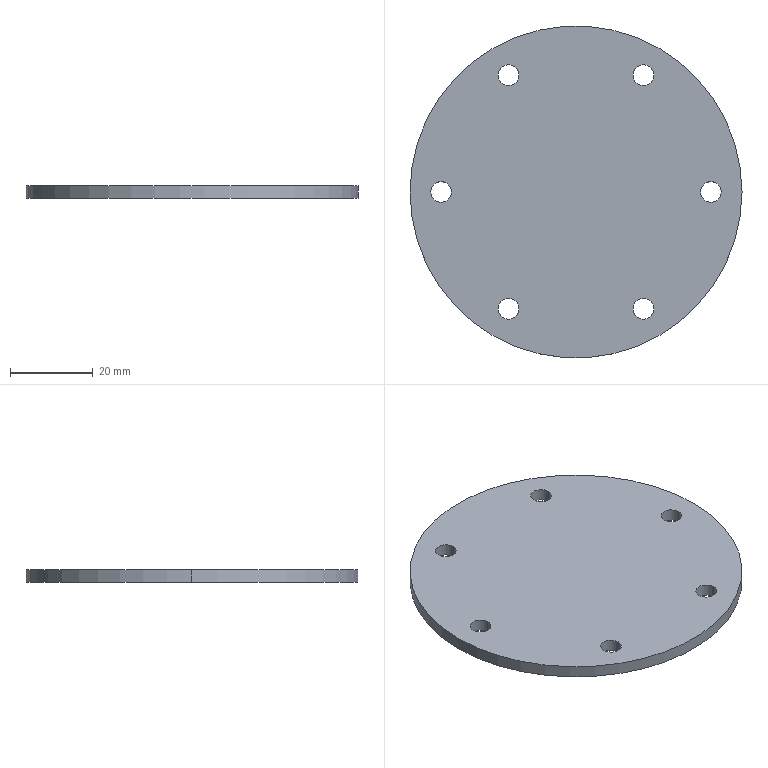Part | SolidWorks | features FlatPattern 1, SMBaseFlange 1, SheetMetal 1 | 1 solid | 16 faces | box 80 x 80 x 3 mm | volume 14726 mm3 | cylinder 14 | plane 2 | commonest cylinder face diameters 5 x12 80 x2
STEP:
#1=CARTESIAN_POINT('',(498.39,-36.604,3.));
#2=VERTEX_POINT('',#1);
#3=CARTESIAN_POINT('',(503.39,-36.604,3.));
#4=VERTEX_POINT('',#3);
#5=CARTESIAN_POINT('',(500.89,-36.604,3.));
#6=DIRECTION('',(0.,0.,1.));
#7=DIRECTION('',(1.,0.,0.));
#8=AXIS2_PLACEMENT_3D('',#5,#6,#7);
#9=CIRCLE('',#8,2.5);
#10=EDGE_CURVE('',#2,#4,#9,.T.);
#11=ORIENTED_EDGE('',*,*,#10,.T.);
#12=CARTESIAN_POINT('',(503.39,-36.604,0.));
#13=VERTEX_POINT('',#12);
#14=CARTESIAN_POINT('',(503.39,-36.604,3.));
#15=DIRECTION('',(0.,0.,-1.));
#16=VECTOR('',#15,1000.);
#17=LINE('',#14,#16);
#18=EDGE_CURVE('',#4,#13,#17,.T.);
#19=ORIENTED_EDGE('',*,*,#18,.T.);
#20=CARTESIAN_POINT('',(498.39,-36.604,0.));
#21=VERTEX_POINT('',#20);
#22=CARTESIAN_POINT('',(500.89,-36.604,0.));
#23=DIRECTION('',(0.,0.,1.));
#24=DIRECTION('',(1.,0.,0.));
#25=AXIS2_PLACEMENT_3D('',#22,#23,#24);
#26=CIRCLE('',#25,2.5);
#27=EDGE_CURVE('',#21,#13,#26,.T.);
#28=ORIENTED_EDGE('',*,*,#27,.F.);
#29=CARTESIAN_POINT('',(498.39,-36.604,3.));
#30=DIRECTION('',(0.,0.,-1.));
#31=VECTOR('',#30,1000.);
#32=LINE('',#29,#31);
#33=EDGE_CURVE('',#2,#21,#32,.T.);
#34=ORIENTED_EDGE('',*,*,#33,.F.);
#35=EDGE_LOOP('',(#11,#19,#28,#34));
#36=FACE_OUTER_BOUND('',#35,.T.);
#37=CARTESIAN_POINT('',(500.89,-36.604,3.));
#38=DIRECTION('',(0.,0.,-1.));
#39=DIRECTION('',(-1.,0.,0.));
#40=AXIS2_PLACEMENT_3D('',#37,#38,#39);
#41=CYLINDRICAL_SURFACE('',#40,2.5);
#42=ADVANCED_FACE('',(#36),#41,.F.);
#43=CARTESIAN_POINT('',(465.89,-36.604,3.));
#44=VERTEX_POINT('',#43);
#45=CARTESIAN_POINT('',(470.89,-36.604,3.));
#46=VERTEX_POINT('',#45);
#47=CARTESIAN_POINT('',(468.39,-36.604,3.));
#48=DIRECTION('',(0.,0.,1.));
#49=DIRECTION('',(1.,0.,0.));
#50=AXIS2_PLACEMENT_3D('',#47,#48,#49);
#51=CIRCLE('',#50,2.5);
#52=EDGE_CURVE('',#44,#46,#51,.T.);
#53=ORIENTED_EDGE('',*,*,#52,.T.);
#54=CARTESIAN_POINT('',(470.89,-36.604,0.));
#55=VERTEX_POINT('',#54);
#56=CARTESIAN_POINT('',(470.89,-36.604,3.));
#57=DIRECTION('',(0.,0.,-1.));
#58=VECTOR('',#57,1000.);
#59=LINE('',#56,#58);
#60=EDGE_CURVE('',#46,#55,#59,.T.);
#61=ORIENTED_EDGE('',*,*,#60,.T.);
#62=CARTESIAN_POINT('',(465.89,-36.604,0.));
#63=VERTEX_POINT('',#62);
#64=CARTESIAN_POINT('',(468.39,-36.604,0.));
#65=DIRECTION('',(0.,0.,1.));
#66=DIRECTION('',(1.,0.,0.));
#67=AXIS2_PLACEMENT_3D('',#64,#65,#66);
#68=CIRCLE('',#67,2.5);
#69=EDGE_CURVE('',#63,#55,#68,.T.);
#70=ORIENTED_EDGE('',*,*,#69,.F.);
#71=CARTESIAN_POINT('',(465.89,-36.604,3.));
#72=DIRECTION('',(0.,0.,-1.));
#73=VECTOR('',#72,1000.);
#74=LINE('',#71,#73);
#75=EDGE_CURVE('',#44,#63,#74,.T.);
#76=ORIENTED_EDGE('',*,*,#75,.F.);
#77=EDGE_LOOP('',(#53,#61,#70,#76));
#78=FACE_OUTER_BOUND('',#77,.T.);
#79=CARTESIAN_POINT('',(468.39,-36.604,3.));
#80=DIRECTION('',(0.,0.,-1.));
#81=DIRECTION('',(-1.,0.,0.));
#82=AXIS2_PLACEMENT_3D('',#79,#80,#81);
#83=CYLINDRICAL_SURFACE('',#82,2.5);
#84=ADVANCED_FACE('',(#78),#83,.F.);
#85=CARTESIAN_POINT('',(449.64,-64.75,3.));
#86=VERTEX_POINT('',#85);
#87=CARTESIAN_POINT('',(454.64,-64.75,3.));
#88=VERTEX_POINT('',#87);
#89=CARTESIAN_POINT('',(452.14,-64.75,3.));
#90=DIRECTION('',(0.,0.,1.));
#91=DIRECTION('',(1.,0.,0.));
#92=AXIS2_PLACEMENT_3D('',#89,#90,#91);
#93=CIRCLE('',#92,2.5);
#94=EDGE_CURVE('',#86,#88,#93,.T.);
#95=ORIENTED_EDGE('',*,*,#94,.T.);
#96=CARTESIAN_POINT('',(454.64,-64.75,0.));
#97=VERTEX_POINT('',#96);
#98=CARTESIAN_POINT('',(454.64,-64.75,3.));
#99=DIRECTION('',(0.,0.,-1.));
#100=VECTOR('',#99,1000.);
#101=LINE('',#98,#100);
#102=EDGE_CURVE('',#88,#97,#101,.T.);
#103=ORIENTED_EDGE('',*,*,#102,.T.);
#104=CARTESIAN_POINT('',(449.64,-64.75,0.));
#105=VERTEX_POINT('',#104);
#106=CARTESIAN_POINT('',(452.14,-64.75,0.));
#107=DIRECTION('',(0.,0.,1.));
#108=DIRECTION('',(1.,0.,0.));
#109=AXIS2_PLACEMENT_3D('',#106,#107,#108);
#110=CIRCLE('',#109,2.5);
#111=EDGE_CURVE('',#105,#97,#110,.T.);
#112=ORIENTED_EDGE('',*,*,#111,.F.);
#113=CARTESIAN_POINT('',(449.64,-64.75,3.));
#114=DIRECTION('',(0.,0.,-1.));
#115=VECTOR('',#114,1000.);
#116=LINE('',#113,#115);
#117=EDGE_CURVE('',#86,#105,#116,.T.);
#118=ORIENTED_EDGE('',*,*,#117,.F.);
#119=EDGE_LOOP('',(#95,#103,#112,#118));
#120=FACE_OUTER_BOUND('',#119,.T.);
#121=CARTESIAN_POINT('',(452.14,-64.75,3.));
#122=DIRECTION('',(0.,0.,-1.));
#123=DIRECTION('',(-1.,0.,0.));
#124=AXIS2_PLACEMENT_3D('',#121,#122,#123);
#125=CYLINDRICAL_SURFACE('',#124,2.5);
#126=ADVANCED_FACE('',(#120),#125,.F.);
#127=CARTESIAN_POINT('',(465.89,-92.896,3.));
#128=VERTEX_POINT('',#127);
#129=CARTESIAN_POINT('',(470.89,-92.896,3.));
#130=VERTEX_POINT('',#129);
#131=CARTESIAN_POINT('',(468.39,-92.896,3.));
#132=DIRECTION('',(0.,0.,1.));
#133=DIRECTION('',(1.,0.,0.));
#134=AXIS2_PLACEMENT_3D('',#131,#132,#133);
#135=CIRCLE('',#134,2.5);
#136=EDGE_CURVE('',#128,#130,#135,.T.);
#137=ORIENTED_EDGE('',*,*,#136,.T.);
#138=CARTESIAN_POINT('',(470.89,-92.896,0.));
#139=VERTEX_POINT('',#138);
#140=CARTESIAN_POINT('',(470.89,-92.896,3.));
#141=DIRECTION('',(0.,0.,-1.));
#142=VECTOR('',#141,1000.);
#143=LINE('',#140,#142);
#144=EDGE_CURVE('',#130,#139,#143,.T.);
#145=ORIENTED_EDGE('',*,*,#144,.T.);
#146=CARTESIAN_POINT('',(465.89,-92.896,0.));
#147=VERTEX_POINT('',#146);
#148=CARTESIAN_POINT('',(468.39,-92.896,0.));
#149=DIRECTION('',(0.,0.,1.));
#150=DIRECTION('',(1.,0.,0.));
#151=AXIS2_PLACEMENT_3D('',#148,#149,#150);
#152=CIRCLE('',#151,2.5);
#153=EDGE_CURVE('',#147,#139,#152,.T.);
#154=ORIENTED_EDGE('',*,*,#153,.F.);
#155=CARTESIAN_POINT('',(465.89,-92.896,3.));
#156=DIRECTION('',(0.,0.,-1.));
#157=VECTOR('',#156,1000.);
#158=LINE('',#155,#157);
#159=EDGE_CURVE('',#128,#147,#158,.T.);
#160=ORIENTED_EDGE('',*,*,#159,.F.);
#161=EDGE_LOOP('',(#137,#145,#154,#160));
#162=FACE_OUTER_BOUND('',#161,.T.);
#163=CARTESIAN_POINT('',(468.39,-92.896,3.));
#164=DIRECTION('',(0.,0.,-1.));
#165=DIRECTION('',(-1.,0.,0.));
#166=AXIS2_PLACEMENT_3D('',#163,#164,#165);
#167=CYLINDRICAL_SURFACE('',#166,2.5);
#168=ADVANCED_FACE('',(#162),#167,.F.);
#169=CARTESIAN_POINT('',(498.39,-92.896,3.));
#170=VERTEX_POINT('',#169);
#171=CARTESIAN_POINT('',(503.39,-92.896,3.));
#172=VERTEX_POINT('',#171);
#173=CARTESIAN_POINT('',(500.89,-92.896,3.));
#174=DIRECTION('',(0.,0.,1.));
#175=DIRECTION('',(1.,0.,0.));
#176=AXIS2_PLACEMENT_3D('',#173,#174,#175);
#177=CIRCLE('',#176,2.5);
#178=EDGE_CURVE('',#170,#172,#177,.T.);
#179=ORIENTED_EDGE('',*,*,#178,.T.);
#180=CARTESIAN_POINT('',(503.39,-92.896,0.));
#181=VERTEX_POINT('',#180);
#182=CARTESIAN_POINT('',(503.39,-92.896,3.));
#183=DIRECTION('',(0.,0.,-1.));
#184=VECTOR('',#183,1000.);
#185=LINE('',#182,#184);
#186=EDGE_CURVE('',#172,#181,#185,.T.);
#187=ORIENTED_EDGE('',*,*,#186,.T.);
#188=CARTESIAN_POINT('',(498.39,-92.896,0.));
#189=VERTEX_POINT('',#188);
#190=CARTESIAN_POINT('',(500.89,-92.896,0.));
#191=DIRECTION('',(0.,0.,1.));
#192=DIRECTION('',(1.,0.,0.));
#193=AXIS2_PLACEMENT_3D('',#190,#191,#192);
#194=CIRCLE('',#193,2.5);
#195=EDGE_CURVE('',#189,#181,#194,.T.);
#196=ORIENTED_EDGE('',*,*,#195,.F.);
#197=CARTESIAN_POINT('',(498.39,-92.896,3.));
#198=DIRECTION('',(0.,0.,-1.));
#199=VECTOR('',#198,1000.);
#200=LINE('',#197,#199);
#201=EDGE_CURVE('',#170,#189,#200,.T.);
#202=ORIENTED_EDGE('',*,*,#201,.F.);
#203=EDGE_LOOP('',(#179,#187,#196,#202));
#204=FACE_OUTER_BOUND('',#203,.T.);
#205=CARTESIAN_POINT('',(500.89,-92.896,3.));
#206=DIRECTION('',(0.,0.,-1.));
#207=DIRECTION('',(-1.,0.,0.));
#208=AXIS2_PLACEMENT_3D('',#205,#206,#207);
#209=CYLINDRICAL_SURFACE('',#208,2.5);
#210=ADVANCED_FACE('',(#204),#209,.F.);
#211=CARTESIAN_POINT('',(514.64,-64.75,3.));
#212=VERTEX_POINT('',#211);
#213=CARTESIAN_POINT('',(519.64,-64.75,3.));
#214=VERTEX_POINT('',#213);
#215=CARTESIAN_POINT('',(517.14,-64.75,3.));
#216=DIRECTION('',(0.,0.,1.));
#217=DIRECTION('',(1.,0.,0.));
#218=AXIS2_PLACEMENT_3D('',#215,#216,#217);
#219=CIRCLE('',#218,2.5);
#220=EDGE_CURVE('',#212,#214,#219,.T.);
#221=ORIENTED_EDGE('',*,*,#220,.T.);
#222=CARTESIAN_POINT('',(519.64,-64.75,0.));
#223=VERTEX_POINT('',#222);
#224=CARTESIAN_POINT('',(519.64,-64.75,3.));
#225=DIRECTION('',(0.,0.,-1.));
#226=VECTOR('',#225,1000.);
#227=LINE('',#224,#226);
#228=EDGE_CURVE('',#214,#223,#227,.T.);
#229=ORIENTED_EDGE('',*,*,#228,.T.);
#230=CARTESIAN_POINT('',(514.64,-64.75,0.));
#231=VERTEX_POINT('',#230);
#232=CARTESIAN_POINT('',(517.14,-64.75,0.));
#233=DIRECTION('',(0.,0.,1.));
#234=DIRECTION('',(1.,0.,0.));
#235=AXIS2_PLACEMENT_3D('',#232,#233,#234);
#236=CIRCLE('',#235,2.5);
#237=EDGE_CURVE('',#231,#223,#236,.T.);
#238=ORIENTED_EDGE('',*,*,#237,.F.);
#239=CARTESIAN_POINT('',(514.64,-64.75,3.));
#240=DIRECTION('',(0.,0.,-1.));
#241=VECTOR('',#240,1000.);
#242=LINE('',#239,#241);
#243=EDGE_CURVE('',#212,#231,#242,.T.);
#244=ORIENTED_EDGE('',*,*,#243,.F.);
#245=EDGE_LOOP('',(#221,#229,#238,#244));
#246=FACE_OUTER_BOUND('',#245,.T.);
#247=CARTESIAN_POINT('',(517.14,-64.75,3.));
#248=DIRECTION('',(0.,0.,-1.));
#249=DIRECTION('',(-1.,0.,0.));
#250=AXIS2_PLACEMENT_3D('',#247,#248,#249);
#251=CYLINDRICAL_SURFACE('',#250,2.5);
#252=ADVANCED_FACE('',(#246),#251,.F.);
#253=CARTESIAN_POINT('',(524.64,-64.75,3.));
#254=VERTEX_POINT('',#253);
#255=CARTESIAN_POINT('',(444.64,-64.75,3.));
#256=VERTEX_POINT('',#255);
#257=CARTESIAN_POINT('',(484.64,-64.75,3.));
#258=DIRECTION('',(0.,0.,1.));
#259=DIRECTION('',(1.,0.,0.));
#260=AXIS2_PLACEMENT_3D('',#257,#258,#259);
#261=CIRCLE('',#260,40.);
#262=EDGE_CURVE('',#254,#256,#261,.T.);
#263=ORIENTED_EDGE('',*,*,#262,.F.);
#264=CARTESIAN_POINT('',(524.64,-64.75,0.));
#265=VERTEX_POINT('',#264);
#266=CARTESIAN_POINT('',(524.64,-64.75,3.));
#267=DIRECTION('',(0.,0.,-1.));
#268=VECTOR('',#267,1000.);
#269=LINE('',#266,#268);
#270=EDGE_CURVE('',#254,#265,#269,.T.);
#271=ORIENTED_EDGE('',*,*,#270,.T.);
#272=CARTESIAN_POINT('',(444.64,-64.75,0.));
#273=VERTEX_POINT('',#272);
#274=CARTESIAN_POINT('',(484.64,-64.75,0.));
#275=DIRECTION('',(0.,0.,1.));
#276=DIRECTION('',(1.,0.,0.));
#277=AXIS2_PLACEMENT_3D('',#274,#275,#276);
#278=CIRCLE('',#277,40.);
#279=EDGE_CURVE('',#265,#273,#278,.T.);
#280=ORIENTED_EDGE('',*,*,#279,.T.);
#281=CARTESIAN_POINT('',(444.64,-64.75,3.));
#282=DIRECTION('',(0.,0.,-1.));
#283=VECTOR('',#282,1000.);
#284=LINE('',#281,#283);
#285=EDGE_CURVE('',#256,#273,#284,.T.);
#286=ORIENTED_EDGE('',*,*,#285,.F.);
#287=EDGE_LOOP('',(#263,#271,#280,#286));
#288=FACE_OUTER_BOUND('',#287,.T.);
#289=CARTESIAN_POINT('',(484.64,-64.75,3.));
#290=DIRECTION('',(0.,0.,-1.));
#291=DIRECTION('',(-1.,0.,0.));
#292=AXIS2_PLACEMENT_3D('',#289,#290,#291);
#293=CYLINDRICAL_SURFACE('',#292,40.);
#294=ADVANCED_FACE('',(#288),#293,.T.);
#295=ORIENTED_EDGE('',*,*,#52,.F.);
#296=CARTESIAN_POINT('',(468.39,-36.604,3.));
#297=DIRECTION('',(0.,0.,1.));
#298=DIRECTION('',(1.,0.,0.));
#299=AXIS2_PLACEMENT_3D('',#296,#297,#298);
#300=CIRCLE('',#299,2.5);
#301=EDGE_CURVE('',#46,#44,#300,.T.);
#302=ORIENTED_EDGE('',*,*,#301,.F.);
#303=EDGE_LOOP('',(#295,#302));
#304=FACE_BOUND('',#303,.T.);
#305=ORIENTED_EDGE('',*,*,#136,.F.);
#306=CARTESIAN_POINT('',(468.39,-92.896,3.));
#307=DIRECTION('',(0.,0.,1.));
#308=DIRECTION('',(1.,0.,0.));
#309=AXIS2_PLACEMENT_3D('',#306,#307,#308);
#310=CIRCLE('',#309,2.5);
#311=EDGE_CURVE('',#130,#128,#310,.T.);
#312=ORIENTED_EDGE('',*,*,#311,.F.);
#313=EDGE_LOOP('',(#305,#312));
#314=FACE_BOUND('',#313,.T.);
#315=ORIENTED_EDGE('',*,*,#220,.F.);
#316=CARTESIAN_POINT('',(517.14,-64.75,3.));
#317=DIRECTION('',(0.,0.,1.));
#318=DIRECTION('',(1.,0.,0.));
#319=AXIS2_PLACEMENT_3D('',#316,#317,#318);
#320=CIRCLE('',#319,2.5);
#321=EDGE_CURVE('',#214,#212,#320,.T.);
#322=ORIENTED_EDGE('',*,*,#321,.F.);
#323=EDGE_LOOP('',(#315,#322));
#324=FACE_BOUND('',#323,.T.);
#325=CARTESIAN_POINT('',(484.64,-64.75,3.));
#326=DIRECTION('',(0.,0.,1.));
#327=DIRECTION('',(1.,0.,0.));
#328=AXIS2_PLACEMENT_3D('',#325,#326,#327);
#329=CIRCLE('',#328,40.);
#330=EDGE_CURVE('',#256,#254,#329,.T.);
#331=ORIENTED_EDGE('',*,*,#330,.T.);
#332=ORIENTED_EDGE('',*,*,#262,.T.);
#333=EDGE_LOOP('',(#331,#332));
#334=FACE_OUTER_BOUND('',#333,.T.);
#335=ORIENTED_EDGE('',*,*,#178,.F.);
#336=CARTESIAN_POINT('',(500.89,-92.896,3.));
#337=DIRECTION('',(0.,0.,1.));
#338=DIRECTION('',(1.,0.,0.));
#339=AXIS2_PLACEMENT_3D('',#336,#337,#338);
#340=CIRCLE('',#339,2.5);
#341=EDGE_CURVE('',#172,#170,#340,.T.);
#342=ORIENTED_EDGE('',*,*,#341,.F.);
#343=EDGE_LOOP('',(#335,#342));
#344=FACE_BOUND('',#343,.T.);
#345=ORIENTED_EDGE('',*,*,#94,.F.);
#346=CARTESIAN_POINT('',(452.14,-64.75,3.));
#347=DIRECTION('',(0.,0.,1.));
#348=DIRECTION('',(1.,0.,0.));
#349=AXIS2_PLACEMENT_3D('',#346,#347,#348);
#350=CIRCLE('',#349,2.5);
#351=EDGE_CURVE('',#88,#86,#350,.T.);
#352=ORIENTED_EDGE('',*,*,#351,.F.);
#353=EDGE_LOOP('',(#345,#352));
#354=FACE_BOUND('',#353,.T.);
#355=ORIENTED_EDGE('',*,*,#10,.F.);
#356=CARTESIAN_POINT('',(500.89,-36.604,3.));
#357=DIRECTION('',(0.,0.,1.));
#358=DIRECTION('',(1.,0.,0.));
#359=AXIS2_PLACEMENT_3D('',#356,#357,#358);
#360=CIRCLE('',#359,2.5);
#361=EDGE_CURVE('',#4,#2,#360,.T.);
#362=ORIENTED_EDGE('',*,*,#361,.F.);
#363=EDGE_LOOP('',(#355,#362));
#364=FACE_BOUND('',#363,.T.);
#365=CARTESIAN_POINT('',(484.64,-64.75,3.));
#366=DIRECTION('',(0.,0.,1.));
#367=DIRECTION('',(1.,0.,0.));
#368=AXIS2_PLACEMENT_3D('',#365,#366,#367);
#369=PLANE('',#368);
#370=ADVANCED_FACE('',(#304,#314,#324,#334,#344,#354,#364),#369,.T.);
#371=CARTESIAN_POINT('',(484.64,-64.75,0.));
#372=DIRECTION('',(0.,0.,1.));
#373=DIRECTION('',(1.,0.,0.));
#374=AXIS2_PLACEMENT_3D('',#371,#372,#373);
#375=CIRCLE('',#374,40.);
#376=EDGE_CURVE('',#273,#265,#375,.T.);
#377=ORIENTED_EDGE('',*,*,#376,.F.);
#378=ORIENTED_EDGE('',*,*,#279,.F.);
#379=EDGE_LOOP('',(#377,#378));
#380=FACE_OUTER_BOUND('',#379,.T.);
#381=ORIENTED_EDGE('',*,*,#237,.T.);
#382=CARTESIAN_POINT('',(517.14,-64.75,0.));
#383=DIRECTION('',(0.,0.,1.));
#384=DIRECTION('',(1.,0.,0.));
#385=AXIS2_PLACEMENT_3D('',#382,#383,#384);
#386=CIRCLE('',#385,2.5);
#387=EDGE_CURVE('',#223,#231,#386,.T.);
#388=ORIENTED_EDGE('',*,*,#387,.T.);
#389=EDGE_LOOP('',(#381,#388));
#390=FACE_BOUND('',#389,.T.);
#391=ORIENTED_EDGE('',*,*,#195,.T.);
#392=CARTESIAN_POINT('',(500.89,-92.896,0.));
#393=DIRECTION('',(0.,0.,1.));
#394=DIRECTION('',(1.,0.,0.));
#395=AXIS2_PLACEMENT_3D('',#392,#393,#394);
#396=CIRCLE('',#395,2.5);
#397=EDGE_CURVE('',#181,#189,#396,.T.);
#398=ORIENTED_EDGE('',*,*,#397,.T.);
#399=EDGE_LOOP('',(#391,#398));
#400=FACE_BOUND('',#399,.T.);
#401=ORIENTED_EDGE('',*,*,#153,.T.);
#402=CARTESIAN_POINT('',(468.39,-92.896,0.));
#403=DIRECTION('',(0.,0.,1.));
#404=DIRECTION('',(1.,0.,0.));
#405=AXIS2_PLACEMENT_3D('',#402,#403,#404);
#406=CIRCLE('',#405,2.5);
#407=EDGE_CURVE('',#139,#147,#406,.T.);
#408=ORIENTED_EDGE('',*,*,#407,.T.);
#409=EDGE_LOOP('',(#401,#408));
#410=FACE_BOUND('',#409,.T.);
#411=ORIENTED_EDGE('',*,*,#111,.T.);
#412=CARTESIAN_POINT('',(452.14,-64.75,0.));
#413=DIRECTION('',(0.,0.,1.));
#414=DIRECTION('',(1.,0.,0.));
#415=AXIS2_PLACEMENT_3D('',#412,#413,#414);
#416=CIRCLE('',#415,2.5);
#417=EDGE_CURVE('',#97,#105,#416,.T.);
#418=ORIENTED_EDGE('',*,*,#417,.T.);
#419=EDGE_LOOP('',(#411,#418));
#420=FACE_BOUND('',#419,.T.);
#421=ORIENTED_EDGE('',*,*,#69,.T.);
#422=CARTESIAN_POINT('',(468.39,-36.604,0.));
#423=DIRECTION('',(0.,0.,1.));
#424=DIRECTION('',(1.,0.,0.));
#425=AXIS2_PLACEMENT_3D('',#422,#423,#424);
#426=CIRCLE('',#425,2.5);
#427=EDGE_CURVE('',#55,#63,#426,.T.);
#428=ORIENTED_EDGE('',*,*,#427,.T.);
#429=EDGE_LOOP('',(#421,#428));
#430=FACE_BOUND('',#429,.T.);
#431=ORIENTED_EDGE('',*,*,#27,.T.);
#432=CARTESIAN_POINT('',(500.89,-36.604,0.));
#433=DIRECTION('',(0.,0.,1.));
#434=DIRECTION('',(1.,0.,0.));
#435=AXIS2_PLACEMENT_3D('',#432,#433,#434);
#436=CIRCLE('',#435,2.5);
#437=EDGE_CURVE('',#13,#21,#436,.T.);
#438=ORIENTED_EDGE('',*,*,#437,.T.);
#439=EDGE_LOOP('',(#431,#438));
#440=FACE_BOUND('',#439,.T.);
#441=CARTESIAN_POINT('',(484.64,-64.75,0.));
#442=DIRECTION('',(0.,0.,1.));
#443=DIRECTION('',(1.,0.,0.));
#444=AXIS2_PLACEMENT_3D('',#441,#442,#443);
#445=PLANE('',#444);
#446=ADVANCED_FACE('',(#380,#390,#400,#410,#420,#430,#440),#445,.F.);
#447=ORIENTED_EDGE('',*,*,#270,.F.);
#448=ORIENTED_EDGE('',*,*,#330,.F.);
#449=ORIENTED_EDGE('',*,*,#285,.T.);
#450=ORIENTED_EDGE('',*,*,#376,.T.);
#451=EDGE_LOOP('',(#447,#448,#449,#450));
#452=FACE_OUTER_BOUND('',#451,.T.);
#453=CARTESIAN_POINT('',(484.64,-64.75,3.));
#454=DIRECTION('',(0.,0.,-1.));
#455=DIRECTION('',(-1.,0.,0.));
#456=AXIS2_PLACEMENT_3D('',#453,#454,#455);
#457=CYLINDRICAL_SURFACE('',#456,40.);
#458=ADVANCED_FACE('',(#452),#457,.T.);
#459=ORIENTED_EDGE('',*,*,#228,.F.);
#460=ORIENTED_EDGE('',*,*,#321,.T.);
#461=ORIENTED_EDGE('',*,*,#243,.T.);
#462=ORIENTED_EDGE('',*,*,#387,.F.);
#463=EDGE_LOOP('',(#459,#460,#461,#462));
#464=FACE_OUTER_BOUND('',#463,.T.);
#465=CARTESIAN_POINT('',(517.14,-64.75,3.));
#466=DIRECTION('',(0.,0.,-1.));
#467=DIRECTION('',(-1.,0.,0.));
#468=AXIS2_PLACEMENT_3D('',#465,#466,#467);
#469=CYLINDRICAL_SURFACE('',#468,2.5);
#470=ADVANCED_FACE('',(#464),#469,.F.);
#471=ORIENTED_EDGE('',*,*,#186,.F.);
#472=ORIENTED_EDGE('',*,*,#341,.T.);
#473=ORIENTED_EDGE('',*,*,#201,.T.);
#474=ORIENTED_EDGE('',*,*,#397,.F.);
#475=EDGE_LOOP('',(#471,#472,#473,#474));
#476=FACE_OUTER_BOUND('',#475,.T.);
#477=CARTESIAN_POINT('',(500.89,-92.896,3.));
#478=DIRECTION('',(0.,0.,-1.));
#479=DIRECTION('',(-1.,0.,0.));
#480=AXIS2_PLACEMENT_3D('',#477,#478,#479);
#481=CYLINDRICAL_SURFACE('',#480,2.5);
#482=ADVANCED_FACE('',(#476),#481,.F.);
#483=ORIENTED_EDGE('',*,*,#144,.F.);
#484=ORIENTED_EDGE('',*,*,#311,.T.);
#485=ORIENTED_EDGE('',*,*,#159,.T.);
#486=ORIENTED_EDGE('',*,*,#407,.F.);
#487=EDGE_LOOP('',(#483,#484,#485,#486));
#488=FACE_OUTER_BOUND('',#487,.T.);
#489=CARTESIAN_POINT('',(468.39,-92.896,3.));
#490=DIRECTION('',(0.,0.,-1.));
#491=DIRECTION('',(-1.,0.,0.));
#492=AXIS2_PLACEMENT_3D('',#489,#490,#491);
#493=CYLINDRICAL_SURFACE('',#492,2.5);
#494=ADVANCED_FACE('',(#488),#493,.F.);
#495=ORIENTED_EDGE('',*,*,#102,.F.);
#496=ORIENTED_EDGE('',*,*,#351,.T.);
#497=ORIENTED_EDGE('',*,*,#117,.T.);
#498=ORIENTED_EDGE('',*,*,#417,.F.);
#499=EDGE_LOOP('',(#495,#496,#497,#498));
#500=FACE_OUTER_BOUND('',#499,.T.);
#501=CARTESIAN_POINT('',(452.14,-64.75,3.));
#502=DIRECTION('',(0.,0.,-1.));
#503=DIRECTION('',(-1.,0.,0.));
#504=AXIS2_PLACEMENT_3D('',#501,#502,#503);
#505=CYLINDRICAL_SURFACE('',#504,2.5);
#506=ADVANCED_FACE('',(#500),#505,.F.);
#507=ORIENTED_EDGE('',*,*,#60,.F.);
#508=ORIENTED_EDGE('',*,*,#301,.T.);
#509=ORIENTED_EDGE('',*,*,#75,.T.);
#510=ORIENTED_EDGE('',*,*,#427,.F.);
#511=EDGE_LOOP('',(#507,#508,#509,#510));
#512=FACE_OUTER_BOUND('',#511,.T.);
#513=CARTESIAN_POINT('',(468.39,-36.604,3.));
#514=DIRECTION('',(0.,0.,-1.));
#515=DIRECTION('',(-1.,0.,0.));
#516=AXIS2_PLACEMENT_3D('',#513,#514,#515);
#517=CYLINDRICAL_SURFACE('',#516,2.5);
#518=ADVANCED_FACE('',(#512),#517,.F.);
#519=ORIENTED_EDGE('',*,*,#18,.F.);
#520=ORIENTED_EDGE('',*,*,#361,.T.);
#521=ORIENTED_EDGE('',*,*,#33,.T.);
#522=ORIENTED_EDGE('',*,*,#437,.F.);
#523=EDGE_LOOP('',(#519,#520,#521,#522));
#524=FACE_OUTER_BOUND('',#523,.T.);
#525=CARTESIAN_POINT('',(500.89,-36.604,3.));
#526=DIRECTION('',(0.,0.,-1.));
#527=DIRECTION('',(-1.,0.,0.));
#528=AXIS2_PLACEMENT_3D('',#525,#526,#527);
#529=CYLINDRICAL_SURFACE('',#528,2.5);
#530=ADVANCED_FACE('',(#524),#529,.F.);
#531=CLOSED_SHELL('',(#42,#84,#126,#168,#210,#252,#294,#370,#446,#458,#470,#482,#494,#506,#518,#530));
#532=MANIFOLD_SOLID_BREP('',#531);
#533=CARTESIAN_POINT('',(0.,0.,0.));
#534=DIRECTION('',(0.,0.,1.));
#535=DIRECTION('',(1.,0.,0.));
#536=AXIS2_PLACEMENT_3D('',#533,#534,#535);
#537=(LENGTH_UNIT()NAMED_UNIT(*)SI_UNIT(.MILLI.,.METRE.));
#538=UNCERTAINTY_MEASURE_WITH_UNIT(LENGTH_MEASURE(0.00001),#537,'','');
#539=(NAMED_UNIT(*)PLANE_ANGLE_UNIT()SI_UNIT($,.RADIAN.));
#540=(NAMED_UNIT(*)SI_UNIT($,.STERADIAN.)SOLID_ANGLE_UNIT());
#541=(GEOMETRIC_REPRESENTATION_CONTEXT(3)GLOBAL_UNCERTAINTY_ASSIGNED_CONTEXT((#538))GLOBAL_UNIT_ASSIGNED_CONTEXT((#537,#539,#540))REPRESENTATION_CONTEXT('',''));
#542=ADVANCED_BREP_SHAPE_REPRESENTATION('',(#532,#536),#541);